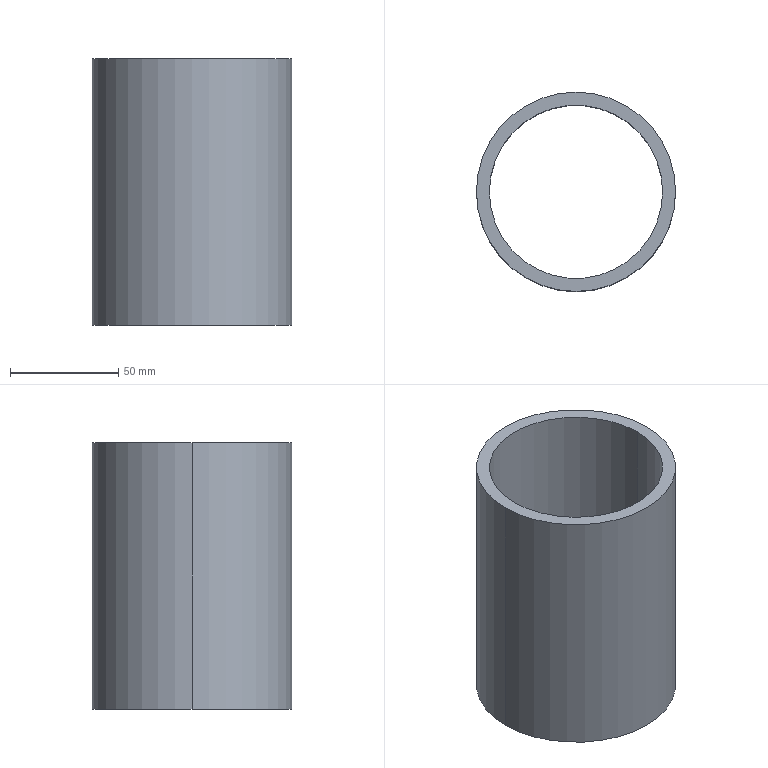Part | NX | features BREP 1 | 1 solid | 6 faces | box 92 x 92 x 123 mm | volume 199391 mm3 | cylinder 4 | plane 2 | commonest cylinder face diameters 80 x2 92 x2
STEP:
#1=CARTESIAN_POINT('',(-40.,0.,123.));
#2=VERTEX_POINT('',#1);
#3=CARTESIAN_POINT('',(40.,0.,123.));
#4=VERTEX_POINT('',#3);
#5=CARTESIAN_POINT('',(0.,0.,123.));
#6=DIRECTION('',(0.,0.,1.));
#7=DIRECTION('',(1.,0.,0.));
#8=AXIS2_PLACEMENT_3D('',#5,#6,#7);
#9=CIRCLE('',#8,40.);
#10=EDGE_CURVE('',#2,#4,#9,.T.);
#11=ORIENTED_EDGE('',*,*,#10,.T.);
#12=CARTESIAN_POINT('',(40.,0.,0.));
#13=VERTEX_POINT('',#12);
#14=CARTESIAN_POINT('',(40.,0.,123.));
#15=DIRECTION('',(0.,0.,-1.));
#16=VECTOR('',#15,1000.);
#17=LINE('',#14,#16);
#18=EDGE_CURVE('',#13,#4,#17,.F.);
#19=ORIENTED_EDGE('',*,*,#18,.F.);
#20=CARTESIAN_POINT('',(-40.,0.,0.));
#21=VERTEX_POINT('',#20);
#22=CARTESIAN_POINT('',(0.,0.,0.));
#23=DIRECTION('',(0.,0.,1.));
#24=DIRECTION('',(1.,0.,0.));
#25=AXIS2_PLACEMENT_3D('',#22,#23,#24);
#26=CIRCLE('',#25,40.);
#27=EDGE_CURVE('',#21,#13,#26,.T.);
#28=ORIENTED_EDGE('',*,*,#27,.F.);
#29=CARTESIAN_POINT('',(-40.,0.,123.));
#30=DIRECTION('',(0.,0.,-1.));
#31=VECTOR('',#30,1000.);
#32=LINE('',#29,#31);
#33=EDGE_CURVE('',#21,#2,#32,.F.);
#34=ORIENTED_EDGE('',*,*,#33,.T.);
#35=EDGE_LOOP('',(#11,#19,#28,#34));
#36=FACE_BOUND('',#35,.T.);
#37=CARTESIAN_POINT('',(0.,0.,123.));
#38=DIRECTION('',(0.,0.,-1.));
#39=DIRECTION('',(1.,0.,0.));
#40=AXIS2_PLACEMENT_3D('',#37,#38,#39);
#41=CYLINDRICAL_SURFACE('',#40,40.);
#42=ADVANCED_FACE('',(#36),#41,.F.);
#43=CARTESIAN_POINT('',(46.,0.,123.));
#44=VERTEX_POINT('',#43);
#45=CARTESIAN_POINT('',(-46.,0.,123.));
#46=VERTEX_POINT('',#45);
#47=CARTESIAN_POINT('',(0.,0.,123.));
#48=DIRECTION('',(0.,0.,1.));
#49=DIRECTION('',(1.,0.,0.));
#50=AXIS2_PLACEMENT_3D('',#47,#48,#49);
#51=CIRCLE('',#50,46.);
#52=EDGE_CURVE('',#44,#46,#51,.T.);
#53=ORIENTED_EDGE('',*,*,#52,.F.);
#54=CARTESIAN_POINT('',(46.,0.,0.));
#55=VERTEX_POINT('',#54);
#56=CARTESIAN_POINT('',(46.,0.,123.));
#57=DIRECTION('',(0.,0.,-1.));
#58=VECTOR('',#57,1000.);
#59=LINE('',#56,#58);
#60=EDGE_CURVE('',#55,#44,#59,.F.);
#61=ORIENTED_EDGE('',*,*,#60,.F.);
#62=CARTESIAN_POINT('',(-46.,0.,0.));
#63=VERTEX_POINT('',#62);
#64=CARTESIAN_POINT('',(0.,0.,0.));
#65=DIRECTION('',(0.,0.,1.));
#66=DIRECTION('',(1.,0.,0.));
#67=AXIS2_PLACEMENT_3D('',#64,#65,#66);
#68=CIRCLE('',#67,46.);
#69=EDGE_CURVE('',#55,#63,#68,.T.);
#70=ORIENTED_EDGE('',*,*,#69,.T.);
#71=CARTESIAN_POINT('',(-46.,0.,123.));
#72=DIRECTION('',(0.,0.,-1.));
#73=VECTOR('',#72,1000.);
#74=LINE('',#71,#73);
#75=EDGE_CURVE('',#63,#46,#74,.F.);
#76=ORIENTED_EDGE('',*,*,#75,.T.);
#77=EDGE_LOOP('',(#53,#61,#70,#76));
#78=FACE_BOUND('',#77,.T.);
#79=CARTESIAN_POINT('',(0.,0.,123.));
#80=DIRECTION('',(0.,0.,-1.));
#81=DIRECTION('',(1.,0.,0.));
#82=AXIS2_PLACEMENT_3D('',#79,#80,#81);
#83=CYLINDRICAL_SURFACE('',#82,46.);
#84=ADVANCED_FACE('',(#78),#83,.T.);
#85=CARTESIAN_POINT('',(0.,0.,123.));
#86=DIRECTION('',(0.,0.,1.));
#87=DIRECTION('',(1.,0.,0.));
#88=AXIS2_PLACEMENT_3D('',#85,#86,#87);
#89=CIRCLE('',#88,46.);
#90=EDGE_CURVE('',#46,#44,#89,.T.);
#91=ORIENTED_EDGE('',*,*,#90,.T.);
#92=ORIENTED_EDGE('',*,*,#52,.T.);
#93=EDGE_LOOP('',(#91,#92));
#94=FACE_BOUND('',#93,.T.);
#95=ORIENTED_EDGE('',*,*,#10,.F.);
#96=CARTESIAN_POINT('',(0.,0.,123.));
#97=DIRECTION('',(0.,0.,1.));
#98=DIRECTION('',(1.,0.,0.));
#99=AXIS2_PLACEMENT_3D('',#96,#97,#98);
#100=CIRCLE('',#99,40.);
#101=EDGE_CURVE('',#4,#2,#100,.T.);
#102=ORIENTED_EDGE('',*,*,#101,.F.);
#103=EDGE_LOOP('',(#95,#102));
#104=FACE_BOUND('',#103,.T.);
#105=CARTESIAN_POINT('',(0.,0.,123.));
#106=DIRECTION('',(0.,0.,1.));
#107=DIRECTION('',(-1.,0.,0.));
#108=AXIS2_PLACEMENT_3D('',#105,#106,#107);
#109=PLANE('',#108);
#110=ADVANCED_FACE('',(#94,#104),#109,.T.);
#111=CARTESIAN_POINT('',(0.,0.,0.));
#112=DIRECTION('',(0.,0.,1.));
#113=DIRECTION('',(1.,0.,0.));
#114=AXIS2_PLACEMENT_3D('',#111,#112,#113);
#115=CIRCLE('',#114,46.);
#116=EDGE_CURVE('',#63,#55,#115,.T.);
#117=ORIENTED_EDGE('',*,*,#116,.F.);
#118=ORIENTED_EDGE('',*,*,#69,.F.);
#119=EDGE_LOOP('',(#117,#118));
#120=FACE_BOUND('',#119,.T.);
#121=ORIENTED_EDGE('',*,*,#27,.T.);
#122=CARTESIAN_POINT('',(0.,0.,0.));
#123=DIRECTION('',(0.,0.,1.));
#124=DIRECTION('',(1.,0.,0.));
#125=AXIS2_PLACEMENT_3D('',#122,#123,#124);
#126=CIRCLE('',#125,40.);
#127=EDGE_CURVE('',#13,#21,#126,.T.);
#128=ORIENTED_EDGE('',*,*,#127,.T.);
#129=EDGE_LOOP('',(#121,#128));
#130=FACE_BOUND('',#129,.T.);
#131=CARTESIAN_POINT('',(0.,0.,0.));
#132=DIRECTION('',(0.,0.,1.));
#133=DIRECTION('',(-1.,0.,0.));
#134=AXIS2_PLACEMENT_3D('',#131,#132,#133);
#135=PLANE('',#134);
#136=ADVANCED_FACE('',(#120,#130),#135,.F.);
#137=ORIENTED_EDGE('',*,*,#60,.T.);
#138=ORIENTED_EDGE('',*,*,#90,.F.);
#139=ORIENTED_EDGE('',*,*,#75,.F.);
#140=ORIENTED_EDGE('',*,*,#116,.T.);
#141=EDGE_LOOP('',(#137,#138,#139,#140));
#142=FACE_BOUND('',#141,.T.);
#143=CARTESIAN_POINT('',(0.,0.,123.));
#144=DIRECTION('',(0.,0.,-1.));
#145=DIRECTION('',(1.,0.,0.));
#146=AXIS2_PLACEMENT_3D('',#143,#144,#145);
#147=CYLINDRICAL_SURFACE('',#146,46.);
#148=ADVANCED_FACE('',(#142),#147,.T.);
#149=ORIENTED_EDGE('',*,*,#18,.T.);
#150=ORIENTED_EDGE('',*,*,#101,.T.);
#151=ORIENTED_EDGE('',*,*,#33,.F.);
#152=ORIENTED_EDGE('',*,*,#127,.F.);
#153=EDGE_LOOP('',(#149,#150,#151,#152));
#154=FACE_BOUND('',#153,.T.);
#155=CARTESIAN_POINT('',(0.,0.,123.));
#156=DIRECTION('',(0.,0.,-1.));
#157=DIRECTION('',(1.,0.,0.));
#158=AXIS2_PLACEMENT_3D('',#155,#156,#157);
#159=CYLINDRICAL_SURFACE('',#158,40.);
#160=ADVANCED_FACE('',(#154),#159,.F.);
#161=CLOSED_SHELL('',(#42,#84,#110,#136,#148,#160));
#162=MANIFOLD_SOLID_BREP('',#161);
#163=(LENGTH_UNIT()NAMED_UNIT(*)SI_UNIT(.MILLI.,.METRE.));
#164=UNCERTAINTY_MEASURE_WITH_UNIT(LENGTH_MEASURE(0.00001),#163,'','');
#165=(NAMED_UNIT(*)PLANE_ANGLE_UNIT()SI_UNIT($,.RADIAN.));
#166=(NAMED_UNIT(*)SI_UNIT($,.STERADIAN.)SOLID_ANGLE_UNIT());
#167=(GEOMETRIC_REPRESENTATION_CONTEXT(3)GLOBAL_UNCERTAINTY_ASSIGNED_CONTEXT((#164))GLOBAL_UNIT_ASSIGNED_CONTEXT((#163,#165,#166))REPRESENTATION_CONTEXT('',''));
#168=ADVANCED_BREP_SHAPE_REPRESENTATION('',(#162),#167);